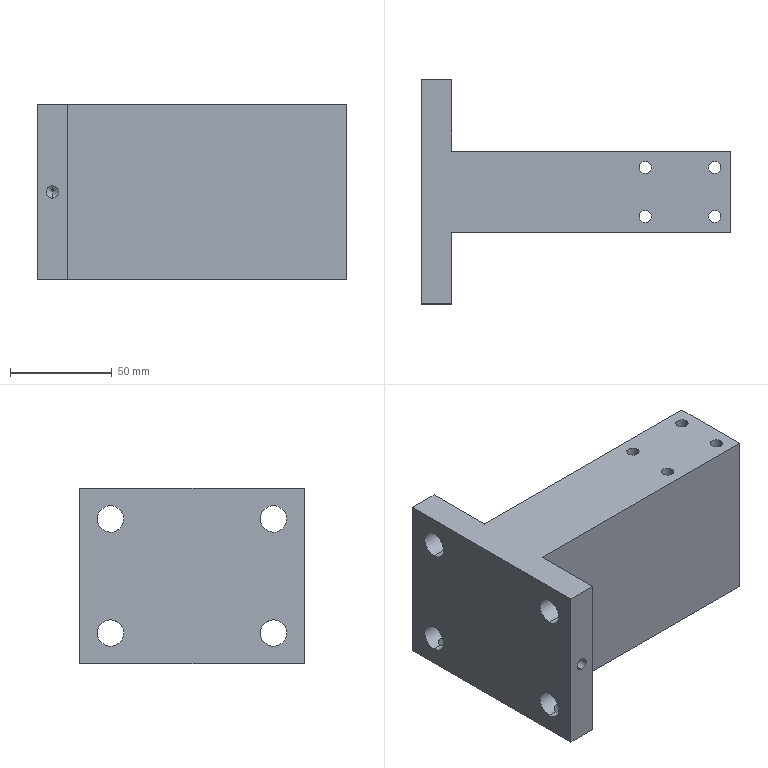Part | STEP file | Positioning_id2126_x_t | 1 solid | 44 faces | box 152 x 110 x 86 mm | volume 594352 mm3 | cylinder 30 | plane 10 | cone 4 | commonest cylinder face diameters 6 x20 13 x8 14 x2